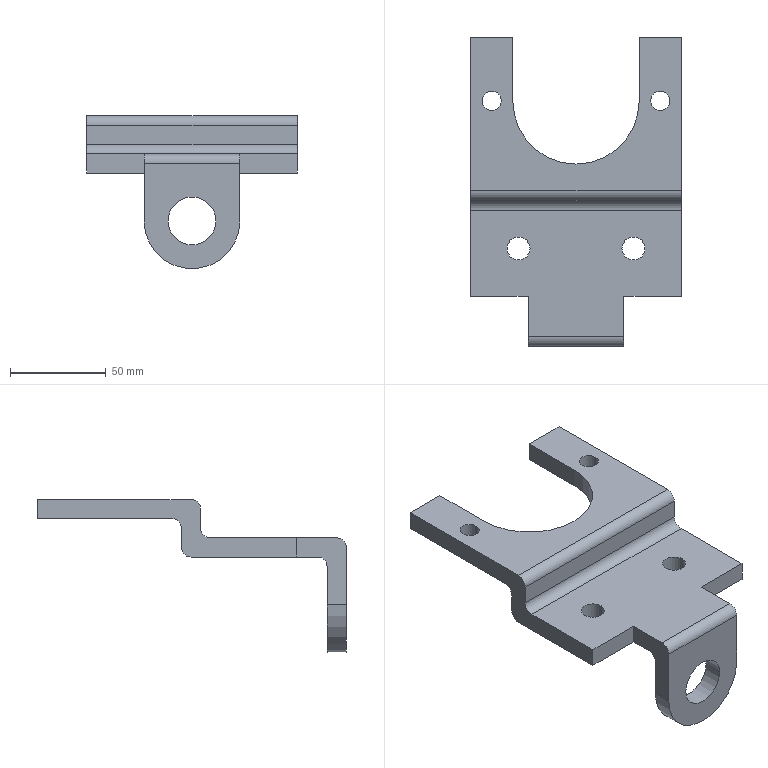Part | SolidWorks | features ICE 4, Fillet 2, Extrusion 1 | 1 solid | 36 faces | box 110 x 161 x 80 mm | volume 158190 mm3 | cylinder 18 | plane 18 | commonest cylinder face diameters 10 x10 12 x4 25 x2 50 x1 66 x1
STEP:
#1=CARTESIAN_POINT('',(-49.,102.,30.));
#2=VERTEX_POINT('',#1);
#3=CARTESIAN_POINT('',(-39.,102.,30.));
#4=VERTEX_POINT('',#3);
#5=CARTESIAN_POINT('',(-44.,102.,30.));
#6=DIRECTION('',(0.,0.,1.));
#7=DIRECTION('',(1.,0.,0.));
#8=AXIS2_PLACEMENT_3D('',#5,#6,#7);
#9=CIRCLE('',#8,5.);
#10=EDGE_CURVE('',#2,#4,#9,.T.);
#11=ORIENTED_EDGE('',*,*,#10,.T.);
#12=CARTESIAN_POINT('',(-39.,102.,20.));
#13=VERTEX_POINT('',#12);
#14=CARTESIAN_POINT('',(-39.,102.,30.));
#15=DIRECTION('',(0.,0.,-1.));
#16=VECTOR('',#15,1000.);
#17=LINE('',#14,#16);
#18=EDGE_CURVE('',#4,#13,#17,.T.);
#19=ORIENTED_EDGE('',*,*,#18,.T.);
#20=CARTESIAN_POINT('',(-49.,102.,20.));
#21=VERTEX_POINT('',#20);
#22=CARTESIAN_POINT('',(-44.,102.,20.));
#23=DIRECTION('',(0.,0.,1.));
#24=DIRECTION('',(1.,0.,0.));
#25=AXIS2_PLACEMENT_3D('',#22,#23,#24);
#26=CIRCLE('',#25,5.);
#27=EDGE_CURVE('',#21,#13,#26,.T.);
#28=ORIENTED_EDGE('',*,*,#27,.F.);
#29=CARTESIAN_POINT('',(-49.,102.,30.));
#30=DIRECTION('',(0.,0.,-1.));
#31=VECTOR('',#30,1000.);
#32=LINE('',#29,#31);
#33=EDGE_CURVE('',#2,#21,#32,.T.);
#34=ORIENTED_EDGE('',*,*,#33,.F.);
#35=EDGE_LOOP('',(#11,#19,#28,#34));
#36=FACE_OUTER_BOUND('',#35,.T.);
#37=CARTESIAN_POINT('',(-44.,102.,30.));
#38=DIRECTION('',(0.,0.,-1.));
#39=DIRECTION('',(-1.,0.,0.));
#40=AXIS2_PLACEMENT_3D('',#37,#38,#39);
#41=CYLINDRICAL_SURFACE('',#40,5.);
#42=ADVANCED_FACE('',(#36),#41,.F.);
#43=CARTESIAN_POINT('',(39.,102.,30.));
#44=VERTEX_POINT('',#43);
#45=CARTESIAN_POINT('',(49.,102.,30.));
#46=VERTEX_POINT('',#45);
#47=CARTESIAN_POINT('',(44.,102.,30.));
#48=DIRECTION('',(0.,0.,1.));
#49=DIRECTION('',(1.,0.,0.));
#50=AXIS2_PLACEMENT_3D('',#47,#48,#49);
#51=CIRCLE('',#50,5.);
#52=EDGE_CURVE('',#44,#46,#51,.T.);
#53=ORIENTED_EDGE('',*,*,#52,.T.);
#54=CARTESIAN_POINT('',(49.,102.,20.));
#55=VERTEX_POINT('',#54);
#56=CARTESIAN_POINT('',(49.,102.,30.));
#57=DIRECTION('',(0.,0.,-1.));
#58=VECTOR('',#57,1000.);
#59=LINE('',#56,#58);
#60=EDGE_CURVE('',#46,#55,#59,.T.);
#61=ORIENTED_EDGE('',*,*,#60,.T.);
#62=CARTESIAN_POINT('',(39.,102.,20.));
#63=VERTEX_POINT('',#62);
#64=CARTESIAN_POINT('',(44.,102.,20.));
#65=DIRECTION('',(0.,0.,1.));
#66=DIRECTION('',(1.,0.,0.));
#67=AXIS2_PLACEMENT_3D('',#64,#65,#66);
#68=CIRCLE('',#67,5.);
#69=EDGE_CURVE('',#63,#55,#68,.T.);
#70=ORIENTED_EDGE('',*,*,#69,.F.);
#71=CARTESIAN_POINT('',(39.,102.,30.));
#72=DIRECTION('',(0.,0.,-1.));
#73=VECTOR('',#72,1000.);
#74=LINE('',#71,#73);
#75=EDGE_CURVE('',#44,#63,#74,.T.);
#76=ORIENTED_EDGE('',*,*,#75,.F.);
#77=EDGE_LOOP('',(#53,#61,#70,#76));
#78=FACE_OUTER_BOUND('',#77,.T.);
#79=CARTESIAN_POINT('',(44.,102.,30.));
#80=DIRECTION('',(0.,0.,-1.));
#81=DIRECTION('',(-1.,0.,0.));
#82=AXIS2_PLACEMENT_3D('',#79,#80,#81);
#83=CYLINDRICAL_SURFACE('',#82,5.);
#84=ADVANCED_FACE('',(#78),#83,.F.);
#85=CARTESIAN_POINT('',(12.5,-26.,-25.));
#86=VERTEX_POINT('',#85);
#87=CARTESIAN_POINT('',(-12.5,-26.,-25.));
#88=VERTEX_POINT('',#87);
#89=CARTESIAN_POINT('',(0.,-26.,-25.));
#90=DIRECTION('',(0.,1.,0.));
#91=DIRECTION('',(-1.,0.,0.));
#92=AXIS2_PLACEMENT_3D('',#89,#90,#91);
#93=CIRCLE('',#92,12.5);
#94=EDGE_CURVE('',#86,#88,#93,.T.);
#95=ORIENTED_EDGE('',*,*,#94,.F.);
#96=CARTESIAN_POINT('',(12.5,-16.,-25.));
#97=VERTEX_POINT('',#96);
#98=CARTESIAN_POINT('',(12.5,-26.,-25.));
#99=DIRECTION('',(0.,1.,0.));
#100=VECTOR('',#99,1000.);
#101=LINE('',#98,#100);
#102=EDGE_CURVE('',#86,#97,#101,.T.);
#103=ORIENTED_EDGE('',*,*,#102,.T.);
#104=CARTESIAN_POINT('',(-12.5,-16.,-25.));
#105=VERTEX_POINT('',#104);
#106=CARTESIAN_POINT('',(0.,-16.,-25.));
#107=DIRECTION('',(0.,1.,0.));
#108=DIRECTION('',(-1.,0.,0.));
#109=AXIS2_PLACEMENT_3D('',#106,#107,#108);
#110=CIRCLE('',#109,12.5);
#111=EDGE_CURVE('',#97,#105,#110,.T.);
#112=ORIENTED_EDGE('',*,*,#111,.T.);
#113=CARTESIAN_POINT('',(-12.5,-26.,-25.));
#114=DIRECTION('',(0.,1.,0.));
#115=VECTOR('',#114,1000.);
#116=LINE('',#113,#115);
#117=EDGE_CURVE('',#88,#105,#116,.T.);
#118=ORIENTED_EDGE('',*,*,#117,.F.);
#119=EDGE_LOOP('',(#95,#103,#112,#118));
#120=FACE_OUTER_BOUND('',#119,.T.);
#121=CARTESIAN_POINT('',(0.,-26.,-25.));
#122=DIRECTION('',(0.,1.,0.));
#123=DIRECTION('',(-1.,0.,0.));
#124=AXIS2_PLACEMENT_3D('',#121,#122,#123);
#125=CYLINDRICAL_SURFACE('',#124,12.5);
#126=ADVANCED_FACE('',(#120),#125,.F.);
#127=CARTESIAN_POINT('',(24.,25.,10.));
#128=VERTEX_POINT('',#127);
#129=CARTESIAN_POINT('',(36.,25.,10.));
#130=VERTEX_POINT('',#129);
#131=CARTESIAN_POINT('',(30.,25.,10.));
#132=DIRECTION('',(0.,0.,1.));
#133=DIRECTION('',(1.,0.,0.));
#134=AXIS2_PLACEMENT_3D('',#131,#132,#133);
#135=CIRCLE('',#134,6.);
#136=EDGE_CURVE('',#128,#130,#135,.T.);
#137=ORIENTED_EDGE('',*,*,#136,.T.);
#138=CARTESIAN_POINT('',(36.,25.,0.));
#139=VERTEX_POINT('',#138);
#140=CARTESIAN_POINT('',(36.,25.,10.));
#141=DIRECTION('',(0.,0.,-1.));
#142=VECTOR('',#141,1000.);
#143=LINE('',#140,#142);
#144=EDGE_CURVE('',#130,#139,#143,.T.);
#145=ORIENTED_EDGE('',*,*,#144,.T.);
#146=CARTESIAN_POINT('',(24.,25.,0.));
#147=VERTEX_POINT('',#146);
#148=CARTESIAN_POINT('',(30.,25.,0.));
#149=DIRECTION('',(0.,0.,1.));
#150=DIRECTION('',(1.,0.,0.));
#151=AXIS2_PLACEMENT_3D('',#148,#149,#150);
#152=CIRCLE('',#151,6.);
#153=EDGE_CURVE('',#147,#139,#152,.T.);
#154=ORIENTED_EDGE('',*,*,#153,.F.);
#155=CARTESIAN_POINT('',(24.,25.,10.));
#156=DIRECTION('',(0.,0.,-1.));
#157=VECTOR('',#156,1000.);
#158=LINE('',#155,#157);
#159=EDGE_CURVE('',#128,#147,#158,.T.);
#160=ORIENTED_EDGE('',*,*,#159,.F.);
#161=EDGE_LOOP('',(#137,#145,#154,#160));
#162=FACE_OUTER_BOUND('',#161,.T.);
#163=CARTESIAN_POINT('',(30.,25.,10.));
#164=DIRECTION('',(0.,0.,-1.));
#165=DIRECTION('',(-1.,0.,0.));
#166=AXIS2_PLACEMENT_3D('',#163,#164,#165);
#167=CYLINDRICAL_SURFACE('',#166,6.);
#168=ADVANCED_FACE('',(#162),#167,.F.);
#169=CARTESIAN_POINT('',(-36.,25.,10.));
#170=VERTEX_POINT('',#169);
#171=CARTESIAN_POINT('',(-24.,25.,10.));
#172=VERTEX_POINT('',#171);
#173=CARTESIAN_POINT('',(-30.,25.,10.));
#174=DIRECTION('',(0.,0.,1.));
#175=DIRECTION('',(1.,0.,0.));
#176=AXIS2_PLACEMENT_3D('',#173,#174,#175);
#177=CIRCLE('',#176,6.);
#178=EDGE_CURVE('',#170,#172,#177,.T.);
#179=ORIENTED_EDGE('',*,*,#178,.T.);
#180=CARTESIAN_POINT('',(-24.,25.,0.));
#181=VERTEX_POINT('',#180);
#182=CARTESIAN_POINT('',(-24.,25.,10.));
#183=DIRECTION('',(0.,0.,-1.));
#184=VECTOR('',#183,1000.);
#185=LINE('',#182,#184);
#186=EDGE_CURVE('',#172,#181,#185,.T.);
#187=ORIENTED_EDGE('',*,*,#186,.T.);
#188=CARTESIAN_POINT('',(-36.,25.,0.));
#189=VERTEX_POINT('',#188);
#190=CARTESIAN_POINT('',(-30.,25.,0.));
#191=DIRECTION('',(0.,0.,1.));
#192=DIRECTION('',(1.,0.,0.));
#193=AXIS2_PLACEMENT_3D('',#190,#191,#192);
#194=CIRCLE('',#193,6.);
#195=EDGE_CURVE('',#189,#181,#194,.T.);
#196=ORIENTED_EDGE('',*,*,#195,.F.);
#197=CARTESIAN_POINT('',(-36.,25.,10.));
#198=DIRECTION('',(0.,0.,-1.));
#199=VECTOR('',#198,1000.);
#200=LINE('',#197,#199);
#201=EDGE_CURVE('',#170,#189,#200,.T.);
#202=ORIENTED_EDGE('',*,*,#201,.F.);
#203=EDGE_LOOP('',(#179,#187,#196,#202));
#204=FACE_OUTER_BOUND('',#203,.T.);
#205=CARTESIAN_POINT('',(-30.,25.,10.));
#206=DIRECTION('',(0.,0.,-1.));
#207=DIRECTION('',(-1.,0.,0.));
#208=AXIS2_PLACEMENT_3D('',#205,#206,#207);
#209=CYLINDRICAL_SURFACE('',#208,6.);
#210=ADVANCED_FACE('',(#204),#209,.F.);
#211=CARTESIAN_POINT('',(25.,-21.,10.));
#212=VERTEX_POINT('',#211);
#213=CARTESIAN_POINT('',(25.,0.,10.));
#214=VERTEX_POINT('',#213);
#215=CARTESIAN_POINT('',(25.,-16.,10.));
#216=DIRECTION('',(0.,1.,0.));
#217=VECTOR('',#216,1000.);
#218=LINE('',#215,#217);
#219=EDGE_CURVE('',#212,#214,#218,.T.);
#220=ORIENTED_EDGE('',*,*,#219,.F.);
#221=CARTESIAN_POINT('',(25.,-26.,5.));
#222=VERTEX_POINT('',#221);
#223=CARTESIAN_POINT('',(25.,-21.,5.));
#224=DIRECTION('',(1.,0.,0.));
#225=DIRECTION('',(0.,0.,1.));
#226=AXIS2_PLACEMENT_3D('',#223,#224,#225);
#227=CIRCLE('',#226,5.);
#228=EDGE_CURVE('',#212,#222,#227,.T.);
#229=ORIENTED_EDGE('',*,*,#228,.T.);
#230=CARTESIAN_POINT('',(25.,-26.,-25.));
#231=VERTEX_POINT('',#230);
#232=CARTESIAN_POINT('',(25.,-26.,-50.));
#233=DIRECTION('',(0.,0.,1.));
#234=VECTOR('',#233,1000.);
#235=LINE('',#232,#234);
#236=EDGE_CURVE('',#231,#222,#235,.T.);
#237=ORIENTED_EDGE('',*,*,#236,.F.);
#238=CARTESIAN_POINT('',(25.,-16.,-25.));
#239=VERTEX_POINT('',#238);
#240=CARTESIAN_POINT('',(25.,-26.,-25.));
#241=DIRECTION('',(0.,1.,0.));
#242=VECTOR('',#241,1000.);
#243=LINE('',#240,#242);
#244=EDGE_CURVE('',#231,#239,#243,.T.);
#245=ORIENTED_EDGE('',*,*,#244,.T.);
#246=CARTESIAN_POINT('',(25.,-16.,-5.));
#247=VERTEX_POINT('',#246);
#248=CARTESIAN_POINT('',(25.,-16.,-50.));
#249=DIRECTION('',(0.,0.,1.));
#250=VECTOR('',#249,1000.);
#251=LINE('',#248,#250);
#252=EDGE_CURVE('',#239,#247,#251,.T.);
#253=ORIENTED_EDGE('',*,*,#252,.T.);
#254=CARTESIAN_POINT('',(25.,-11.,0.));
#255=VERTEX_POINT('',#254);
#256=CARTESIAN_POINT('',(25.,-11.,-5.));
#257=DIRECTION('',(-1.,0.,0.));
#258=DIRECTION('',(0.,0.,1.));
#259=AXIS2_PLACEMENT_3D('',#256,#257,#258);
#260=CIRCLE('',#259,5.);
#261=EDGE_CURVE('',#247,#255,#260,.T.);
#262=ORIENTED_EDGE('',*,*,#261,.T.);
#263=CARTESIAN_POINT('',(25.,0.,0.));
#264=VERTEX_POINT('',#263);
#265=CARTESIAN_POINT('',(25.,-16.,0.));
#266=DIRECTION('',(0.,1.,0.));
#267=VECTOR('',#266,1000.);
#268=LINE('',#265,#267);
#269=EDGE_CURVE('',#255,#264,#268,.T.);
#270=ORIENTED_EDGE('',*,*,#269,.T.);
#271=CARTESIAN_POINT('',(25.,0.,10.));
#272=DIRECTION('',(0.,0.,-1.));
#273=VECTOR('',#272,1000.);
#274=LINE('',#271,#273);
#275=EDGE_CURVE('',#214,#264,#274,.T.);
#276=ORIENTED_EDGE('',*,*,#275,.F.);
#277=EDGE_LOOP('',(#220,#229,#237,#245,#253,#262,#270,#276));
#278=FACE_OUTER_BOUND('',#277,.T.);
#279=CARTESIAN_POINT('',(25.,-16.,10.));
#280=DIRECTION('',(-1.,0.,0.));
#281=DIRECTION('',(0.,0.,1.));
#282=AXIS2_PLACEMENT_3D('',#279,#280,#281);
#283=PLANE('',#282);
#284=ADVANCED_FACE('',(#278),#283,.F.);
#285=ORIENTED_EDGE('',*,*,#178,.F.);
#286=CARTESIAN_POINT('',(-30.,25.,10.));
#287=DIRECTION('',(0.,0.,1.));
#288=DIRECTION('',(1.,0.,0.));
#289=AXIS2_PLACEMENT_3D('',#286,#287,#288);
#290=CIRCLE('',#289,6.);
#291=EDGE_CURVE('',#172,#170,#290,.T.);
#292=ORIENTED_EDGE('',*,*,#291,.F.);
#293=EDGE_LOOP('',(#285,#292));
#294=FACE_BOUND('',#293,.T.);
#295=CARTESIAN_POINT('',(55.,0.,10.));
#296=VERTEX_POINT('',#295);
#297=CARTESIAN_POINT('',(55.,45.,10.));
#298=VERTEX_POINT('',#297);
#299=CARTESIAN_POINT('',(55.,50.,10.));
#300=DIRECTION('',(0.,1.,0.));
#301=VECTOR('',#300,1000.);
#302=LINE('',#299,#301);
#303=EDGE_CURVE('',#296,#298,#302,.T.);
#304=ORIENTED_EDGE('',*,*,#303,.T.);
#305=CARTESIAN_POINT('',(-55.,45.,10.));
#306=VERTEX_POINT('',#305);
#307=CARTESIAN_POINT('',(0.,45.,10.));
#308=DIRECTION('',(-1.,0.,0.));
#309=VECTOR('',#308,1000.);
#310=LINE('',#307,#309);
#311=EDGE_CURVE('',#298,#306,#310,.T.);
#312=ORIENTED_EDGE('',*,*,#311,.T.);
#313=CARTESIAN_POINT('',(-55.,0.,10.));
#314=VERTEX_POINT('',#313);
#315=CARTESIAN_POINT('',(-55.,50.,10.));
#316=DIRECTION('',(0.,-1.,0.));
#317=VECTOR('',#316,1000.);
#318=LINE('',#315,#317);
#319=EDGE_CURVE('',#306,#314,#318,.T.);
#320=ORIENTED_EDGE('',*,*,#319,.T.);
#321=CARTESIAN_POINT('',(-25.,0.,10.));
#322=VERTEX_POINT('',#321);
#323=CARTESIAN_POINT('',(-55.,0.,10.));
#324=DIRECTION('',(1.,0.,0.));
#325=VECTOR('',#324,1000.);
#326=LINE('',#323,#325);
#327=EDGE_CURVE('',#314,#322,#326,.T.);
#328=ORIENTED_EDGE('',*,*,#327,.T.);
#329=CARTESIAN_POINT('',(-25.,-21.,10.));
#330=VERTEX_POINT('',#329);
#331=CARTESIAN_POINT('',(-25.,0.,10.));
#332=DIRECTION('',(0.,-1.,0.));
#333=VECTOR('',#332,1000.);
#334=LINE('',#331,#333);
#335=EDGE_CURVE('',#322,#330,#334,.T.);
#336=ORIENTED_EDGE('',*,*,#335,.T.);
#337=CARTESIAN_POINT('',(25.,-21.,10.));
#338=DIRECTION('',(1.,0.,0.));
#339=VECTOR('',#338,1000.);
#340=LINE('',#337,#339);
#341=EDGE_CURVE('',#330,#212,#340,.T.);
#342=ORIENTED_EDGE('',*,*,#341,.T.);
#343=ORIENTED_EDGE('',*,*,#219,.T.);
#344=CARTESIAN_POINT('',(55.,0.,10.));
#345=DIRECTION('',(1.,0.,0.));
#346=VECTOR('',#345,1000.);
#347=LINE('',#344,#346);
#348=EDGE_CURVE('',#214,#296,#347,.T.);
#349=ORIENTED_EDGE('',*,*,#348,.T.);
#350=EDGE_LOOP('',(#304,#312,#320,#328,#336,#342,#343,#349));
#351=FACE_OUTER_BOUND('',#350,.T.);
#352=ORIENTED_EDGE('',*,*,#136,.F.);
#353=CARTESIAN_POINT('',(30.,25.,10.));
#354=DIRECTION('',(0.,0.,1.));
#355=DIRECTION('',(1.,0.,0.));
#356=AXIS2_PLACEMENT_3D('',#353,#354,#355);
#357=CIRCLE('',#356,6.);
#358=EDGE_CURVE('',#130,#128,#357,.T.);
#359=ORIENTED_EDGE('',*,*,#358,.F.);
#360=EDGE_LOOP('',(#352,#359));
#361=FACE_BOUND('',#360,.T.);
#362=CARTESIAN_POINT('',(0.,0.,10.));
#363=DIRECTION('',(0.,0.,-1.));
#364=DIRECTION('',(-1.,0.,0.));
#365=AXIS2_PLACEMENT_3D('',#362,#363,#364);
#366=PLANE('',#365);
#367=ADVANCED_FACE('',(#294,#351,#361),#366,.F.);
#368=ORIENTED_EDGE('',*,*,#195,.T.);
#369=CARTESIAN_POINT('',(-30.,25.,0.));
#370=DIRECTION('',(0.,0.,1.));
#371=DIRECTION('',(1.,0.,0.));
#372=AXIS2_PLACEMENT_3D('',#369,#370,#371);
#373=CIRCLE('',#372,6.);
#374=EDGE_CURVE('',#181,#189,#373,.T.);
#375=ORIENTED_EDGE('',*,*,#374,.T.);
#376=EDGE_LOOP('',(#368,#375));
#377=FACE_BOUND('',#376,.T.);
#378=CARTESIAN_POINT('',(-55.,55.,0.));
#379=VERTEX_POINT('',#378);
#380=CARTESIAN_POINT('',(-55.,0.,0.));
#381=VERTEX_POINT('',#380);
#382=CARTESIAN_POINT('',(-55.,50.,0.));
#383=DIRECTION('',(0.,-1.,0.));
#384=VECTOR('',#383,1000.);
#385=LINE('',#382,#384);
#386=EDGE_CURVE('',#379,#381,#385,.T.);
#387=ORIENTED_EDGE('',*,*,#386,.F.);
#388=CARTESIAN_POINT('',(55.,55.,0.));
#389=VERTEX_POINT('',#388);
#390=CARTESIAN_POINT('',(0.,55.,0.));
#391=DIRECTION('',(1.,0.,0.));
#392=VECTOR('',#391,1000.);
#393=LINE('',#390,#392);
#394=EDGE_CURVE('',#379,#389,#393,.T.);
#395=ORIENTED_EDGE('',*,*,#394,.T.);
#396=CARTESIAN_POINT('',(55.,0.,0.));
#397=VERTEX_POINT('',#396);
#398=CARTESIAN_POINT('',(55.,50.,0.));
#399=DIRECTION('',(0.,1.,0.));
#400=VECTOR('',#399,1000.);
#401=LINE('',#398,#400);
#402=EDGE_CURVE('',#397,#389,#401,.T.);
#403=ORIENTED_EDGE('',*,*,#402,.F.);
#404=CARTESIAN_POINT('',(25.,0.,0.));
#405=DIRECTION('',(1.,0.,0.));
#406=VECTOR('',#405,1000.);
#407=LINE('',#404,#406);
#408=EDGE_CURVE('',#264,#397,#407,.T.);
#409=ORIENTED_EDGE('',*,*,#408,.F.);
#410=ORIENTED_EDGE('',*,*,#269,.F.);
#411=CARTESIAN_POINT('',(-25.,-11.,0.));
#412=VERTEX_POINT('',#411);
#413=CARTESIAN_POINT('',(-25.,-11.,0.));
#414=DIRECTION('',(-1.,0.,0.));
#415=VECTOR('',#414,1000.);
#416=LINE('',#413,#415);
#417=EDGE_CURVE('',#255,#412,#416,.T.);
#418=ORIENTED_EDGE('',*,*,#417,.T.);
#419=CARTESIAN_POINT('',(-25.,0.,0.));
#420=VERTEX_POINT('',#419);
#421=CARTESIAN_POINT('',(-25.,0.,0.));
#422=DIRECTION('',(0.,-1.,0.));
#423=VECTOR('',#422,1000.);
#424=LINE('',#421,#423);
#425=EDGE_CURVE('',#420,#412,#424,.T.);
#426=ORIENTED_EDGE('',*,*,#425,.F.);
#427=CARTESIAN_POINT('',(-55.,0.,0.));
#428=DIRECTION('',(1.,0.,0.));
#429=VECTOR('',#428,1000.);
#430=LINE('',#427,#429);
#431=EDGE_CURVE('',#381,#420,#430,.T.);
#432=ORIENTED_EDGE('',*,*,#431,.F.);
#433=EDGE_LOOP('',(#387,#395,#403,#409,#410,#418,#426,#432));
#434=FACE_OUTER_BOUND('',#433,.T.);
#435=ORIENTED_EDGE('',*,*,#153,.T.);
#436=CARTESIAN_POINT('',(30.,25.,0.));
#437=DIRECTION('',(0.,0.,1.));
#438=DIRECTION('',(1.,0.,0.));
#439=AXIS2_PLACEMENT_3D('',#436,#437,#438);
#440=CIRCLE('',#439,6.);
#441=EDGE_CURVE('',#139,#147,#440,.T.);
#442=ORIENTED_EDGE('',*,*,#441,.T.);
#443=EDGE_LOOP('',(#435,#442));
#444=FACE_BOUND('',#443,.T.);
#445=CARTESIAN_POINT('',(0.,0.,0.));
#446=DIRECTION('',(0.,0.,-1.));
#447=DIRECTION('',(-1.,0.,0.));
#448=AXIS2_PLACEMENT_3D('',#445,#446,#447);
#449=PLANE('',#448);
#450=ADVANCED_FACE('',(#377,#434,#444),#449,.T.);
#451=CARTESIAN_POINT('',(55.,55.,30.));
#452=VERTEX_POINT('',#451);
#453=CARTESIAN_POINT('',(55.,135.,30.));
#454=VERTEX_POINT('',#453);
#455=CARTESIAN_POINT('',(55.,50.,30.));
#456=DIRECTION('',(0.,1.,0.));
#457=VECTOR('',#456,1000.);
#458=LINE('',#455,#457);
#459=EDGE_CURVE('',#452,#454,#458,.T.);
#460=ORIENTED_EDGE('',*,*,#459,.F.);
#461=CARTESIAN_POINT('',(55.,50.,25.));
#462=VERTEX_POINT('',#461);
#463=CARTESIAN_POINT('',(55.,55.,25.));
#464=DIRECTION('',(1.,0.,0.));
#465=DIRECTION('',(0.,-1.,0.));
#466=AXIS2_PLACEMENT_3D('',#463,#464,#465);
#467=CIRCLE('',#466,5.);
#468=EDGE_CURVE('',#452,#462,#467,.T.);
#469=ORIENTED_EDGE('',*,*,#468,.T.);
#470=CARTESIAN_POINT('',(55.,50.,15.));
#471=VERTEX_POINT('',#470);
#472=CARTESIAN_POINT('',(55.,50.,0.));
#473=DIRECTION('',(0.,0.,1.));
#474=VECTOR('',#473,1000.);
#475=LINE('',#472,#474);
#476=EDGE_CURVE('',#471,#462,#475,.T.);
#477=ORIENTED_EDGE('',*,*,#476,.F.);
#478=CARTESIAN_POINT('',(55.,45.,15.));
#479=DIRECTION('',(-1.,0.,0.));
#480=DIRECTION('',(0.,-1.,0.));
#481=AXIS2_PLACEMENT_3D('',#478,#479,#480);
#482=CIRCLE('',#481,5.);
#483=EDGE_CURVE('',#471,#298,#482,.T.);
#484=ORIENTED_EDGE('',*,*,#483,.T.);
#485=ORIENTED_EDGE('',*,*,#303,.F.);
#486=CARTESIAN_POINT('',(55.,0.,10.));
#487=DIRECTION('',(0.,0.,-1.));
#488=VECTOR('',#487,1000.);
#489=LINE('',#486,#488);
#490=EDGE_CURVE('',#296,#397,#489,.T.);
#491=ORIENTED_EDGE('',*,*,#490,.T.);
#492=ORIENTED_EDGE('',*,*,#402,.T.);
#493=CARTESIAN_POINT('',(55.,60.,5.));
#494=VERTEX_POINT('',#493);
#495=CARTESIAN_POINT('',(55.,55.,5.));
#496=DIRECTION('',(1.,0.,0.));
#497=DIRECTION('',(0.,-1.,0.));
#498=AXIS2_PLACEMENT_3D('',#495,#496,#497);
#499=CIRCLE('',#498,5.);
#500=EDGE_CURVE('',#389,#494,#499,.T.);
#501=ORIENTED_EDGE('',*,*,#500,.T.);
#502=CARTESIAN_POINT('',(55.,60.,15.));
#503=VERTEX_POINT('',#502);
#504=CARTESIAN_POINT('',(55.,60.,0.));
#505=DIRECTION('',(0.,0.,1.));
#506=VECTOR('',#505,1000.);
#507=LINE('',#504,#506);
#508=EDGE_CURVE('',#494,#503,#507,.T.);
#509=ORIENTED_EDGE('',*,*,#508,.T.);
#510=CARTESIAN_POINT('',(55.,65.,20.));
#511=VERTEX_POINT('',#510);
#512=CARTESIAN_POINT('',(55.,65.,15.));
#513=DIRECTION('',(-1.,0.,0.));
#514=DIRECTION('',(0.,-1.,0.));
#515=AXIS2_PLACEMENT_3D('',#512,#513,#514);
#516=CIRCLE('',#515,5.);
#517=EDGE_CURVE('',#503,#511,#516,.T.);
#518=ORIENTED_EDGE('',*,*,#517,.T.);
#519=CARTESIAN_POINT('',(55.,135.,20.));
#520=VERTEX_POINT('',#519);
#521=CARTESIAN_POINT('',(55.,60.,20.));
#522=DIRECTION('',(0.,1.,0.));
#523=VECTOR('',#522,1000.);
#524=LINE('',#521,#523);
#525=EDGE_CURVE('',#511,#520,#524,.T.);
#526=ORIENTED_EDGE('',*,*,#525,.T.);
#527=CARTESIAN_POINT('',(55.,135.,30.));
#528=DIRECTION('',(0.,0.,-1.));
#529=VECTOR('',#528,1000.);
#530=LINE('',#527,#529);
#531=EDGE_CURVE('',#454,#520,#530,.T.);
#532=ORIENTED_EDGE('',*,*,#531,.F.);
#533=EDGE_LOOP('',(#460,#469,#477,#484,#485,#491,#492,#501,#509,#518,#526,#532));
#534=FACE_OUTER_BOUND('',#533,.T.);
#535=CARTESIAN_POINT('',(55.,50.,10.));
#536=DIRECTION('',(-1.,0.,0.));
#537=DIRECTION('',(0.,-1.,0.));
#538=AXIS2_PLACEMENT_3D('',#535,#536,#537);
#539=PLANE('',#538);
#540=ADVANCED_FACE('',(#534),#539,.F.);
#541=CARTESIAN_POINT('',(-55.,50.,15.));
#542=VERTEX_POINT('',#541);
#543=CARTESIAN_POINT('',(-55.,50.,25.));
#544=VERTEX_POINT('',#543);
#545=CARTESIAN_POINT('',(-55.,50.,0.));
#546=DIRECTION('',(0.,0.,1.));
#547=VECTOR('',#546,1000.);
#548=LINE('',#545,#547);
#549=EDGE_CURVE('',#542,#544,#548,.T.);
#550=ORIENTED_EDGE('',*,*,#549,.T.);
#551=CARTESIAN_POINT('',(-55.,55.,30.));
#552=VERTEX_POINT('',#551);
#553=CARTESIAN_POINT('',(-55.,55.,25.));
#554=DIRECTION('',(-1.,0.,0.));
#555=DIRECTION('',(0.,1.,0.));
#556=AXIS2_PLACEMENT_3D('',#553,#554,#555);
#557=CIRCLE('',#556,5.);
#558=EDGE_CURVE('',#544,#552,#557,.T.);
#559=ORIENTED_EDGE('',*,*,#558,.T.);
#560=CARTESIAN_POINT('',(-55.,135.,30.));
#561=VERTEX_POINT('',#560);
#562=CARTESIAN_POINT('',(-55.,60.,30.));
#563=DIRECTION('',(0.,-1.,0.));
#564=VECTOR('',#563,1000.);
#565=LINE('',#562,#564);
#566=EDGE_CURVE('',#561,#552,#565,.T.);
#567=ORIENTED_EDGE('',*,*,#566,.F.);
#568=CARTESIAN_POINT('',(-55.,135.,20.));
#569=VERTEX_POINT('',#568);
#570=CARTESIAN_POINT('',(-55.,135.,30.));
#571=DIRECTION('',(0.,0.,-1.));
#572=VECTOR('',#571,1000.);
#573=LINE('',#570,#572);
#574=EDGE_CURVE('',#561,#569,#573,.T.);
#575=ORIENTED_EDGE('',*,*,#574,.T.);
#576=CARTESIAN_POINT('',(-55.,65.,20.));
#577=VERTEX_POINT('',#576);
#578=CARTESIAN_POINT('',(-55.,60.,20.));
#579=DIRECTION('',(0.,-1.,0.));
#580=VECTOR('',#579,1000.);
#581=LINE('',#578,#580);
#582=EDGE_CURVE('',#569,#577,#581,.T.);
#583=ORIENTED_EDGE('',*,*,#582,.T.);
#584=CARTESIAN_POINT('',(-55.,60.,15.));
#585=VERTEX_POINT('',#584);
#586=CARTESIAN_POINT('',(-55.,65.,15.));
#587=DIRECTION('',(1.,0.,0.));
#588=DIRECTION('',(0.,1.,0.));
#589=AXIS2_PLACEMENT_3D('',#586,#587,#588);
#590=CIRCLE('',#589,5.);
#591=EDGE_CURVE('',#577,#585,#590,.T.);
#592=ORIENTED_EDGE('',*,*,#591,.T.);
#593=CARTESIAN_POINT('',(-55.,60.,5.));
#594=VERTEX_POINT('',#593);
#595=CARTESIAN_POINT('',(-55.,60.,0.));
#596=DIRECTION('',(0.,0.,1.));
#597=VECTOR('',#596,1000.);
#598=LINE('',#595,#597);
#599=EDGE_CURVE('',#594,#585,#598,.T.);
#600=ORIENTED_EDGE('',*,*,#599,.F.);
#601=CARTESIAN_POINT('',(-55.,55.,5.));
#602=DIRECTION('',(-1.,0.,0.));
#603=DIRECTION('',(0.,1.,0.));
#604=AXIS2_PLACEMENT_3D('',#601,#602,#603);
#605=CIRCLE('',#604,5.);
#606=EDGE_CURVE('',#594,#379,#605,.T.);
#607=ORIENTED_EDGE('',*,*,#606,.T.);
#608=ORIENTED_EDGE('',*,*,#386,.T.);
#609=CARTESIAN_POINT('',(-55.,0.,10.));
#610=DIRECTION('',(0.,0.,-1.));
#611=VECTOR('',#610,1000.);
#612=LINE('',#609,#611);
#613=EDGE_CURVE('',#314,#381,#612,.T.);
#614=ORIENTED_EDGE('',*,*,#613,.F.);
#615=ORIENTED_EDGE('',*,*,#319,.F.);
#616=CARTESIAN_POINT('',(-55.,45.,15.));
#617=DIRECTION('',(1.,0.,0.));
#618=DIRECTION('',(0.,1.,0.));
#619=AXIS2_PLACEMENT_3D('',#616,#617,#618);
#620=CIRCLE('',#619,5.);
#621=EDGE_CURVE('',#306,#542,#620,.T.);
#622=ORIENTED_EDGE('',*,*,#621,.T.);
#623=EDGE_LOOP('',(#550,#559,#567,#575,#583,#592,#600,#607,#608,#614,#615,#622));
#624=FACE_OUTER_BOUND('',#623,.T.);
#625=CARTESIAN_POINT('',(-55.,50.,10.));
#626=DIRECTION('',(1.,0.,0.));
#627=DIRECTION('',(0.,1.,0.));
#628=AXIS2_PLACEMENT_3D('',#625,#626,#627);
#629=PLANE('',#628);
#630=ADVANCED_FACE('',(#624),#629,.F.);
#631=ORIENTED_EDGE('',*,*,#431,.T.);
#632=CARTESIAN_POINT('',(-25.,0.,10.));
#633=DIRECTION('',(0.,0.,-1.));
#634=VECTOR('',#633,1000.);
#635=LINE('',#632,#634);
#636=EDGE_CURVE('',#322,#420,#635,.T.);
#637=ORIENTED_EDGE('',*,*,#636,.F.);
#638=ORIENTED_EDGE('',*,*,#327,.F.);
#639=ORIENTED_EDGE('',*,*,#613,.T.);
#640=EDGE_LOOP('',(#631,#637,#638,#639));
#641=FACE_OUTER_BOUND('',#640,.T.);
#642=CARTESIAN_POINT('',(-55.,0.,10.));
#643=DIRECTION('',(0.,1.,0.));
#644=DIRECTION('',(-1.,0.,0.));
#645=AXIS2_PLACEMENT_3D('',#642,#643,#644);
#646=PLANE('',#645);
#647=ADVANCED_FACE('',(#641),#646,.F.);
#648=CARTESIAN_POINT('',(-25.,-26.,-25.));
#649=VERTEX_POINT('',#648);
#650=CARTESIAN_POINT('',(-25.,-26.,5.));
#651=VERTEX_POINT('',#650);
#652=CARTESIAN_POINT('',(-25.,-26.,-50.));
#653=DIRECTION('',(0.,0.,1.));
#654=VECTOR('',#653,1000.);
#655=LINE('',#652,#654);
#656=EDGE_CURVE('',#649,#651,#655,.T.);
#657=ORIENTED_EDGE('',*,*,#656,.T.);
#658=CARTESIAN_POINT('',(-25.,-21.,5.));
#659=DIRECTION('',(-1.,0.,0.));
#660=DIRECTION('',(0.,1.,0.));
#661=AXIS2_PLACEMENT_3D('',#658,#659,#660);
#662=CIRCLE('',#661,5.);
#663=EDGE_CURVE('',#651,#330,#662,.T.);
#664=ORIENTED_EDGE('',*,*,#663,.T.);
#665=ORIENTED_EDGE('',*,*,#335,.F.);
#666=ORIENTED_EDGE('',*,*,#636,.T.);
#667=ORIENTED_EDGE('',*,*,#425,.T.);
#668=CARTESIAN_POINT('',(-25.,-16.,-5.));
#669=VERTEX_POINT('',#668);
#670=CARTESIAN_POINT('',(-25.,-11.,-5.));
#671=DIRECTION('',(1.,0.,0.));
#672=DIRECTION('',(0.,1.,0.));
#673=AXIS2_PLACEMENT_3D('',#670,#671,#672);
#674=CIRCLE('',#673,5.);
#675=EDGE_CURVE('',#412,#669,#674,.T.);
#676=ORIENTED_EDGE('',*,*,#675,.T.);
#677=CARTESIAN_POINT('',(-25.,-16.,-25.));
#678=VERTEX_POINT('',#677);
#679=CARTESIAN_POINT('',(-25.,-16.,-50.));
#680=DIRECTION('',(0.,0.,1.));
#681=VECTOR('',#680,1000.);
#682=LINE('',#679,#681);
#683=EDGE_CURVE('',#678,#669,#682,.T.);
#684=ORIENTED_EDGE('',*,*,#683,.F.);
#685=CARTESIAN_POINT('',(-25.,-26.,-25.));
#686=DIRECTION('',(0.,1.,0.));
#687=VECTOR('',#686,1000.);
#688=LINE('',#685,#687);
#689=EDGE_CURVE('',#649,#678,#688,.T.);
#690=ORIENTED_EDGE('',*,*,#689,.F.);
#691=EDGE_LOOP('',(#657,#664,#665,#666,#667,#676,#684,#690));
#692=FACE_OUTER_BOUND('',#691,.T.);
#693=CARTESIAN_POINT('',(-25.,0.,10.));
#694=DIRECTION('',(1.,0.,0.));
#695=DIRECTION('',(0.,1.,0.));
#696=AXIS2_PLACEMENT_3D('',#693,#694,#695);
#697=PLANE('',#696);
#698=ADVANCED_FACE('',(#692),#697,.F.);
#699=ORIENTED_EDGE('',*,*,#408,.T.);
#700=ORIENTED_EDGE('',*,*,#490,.F.);
#701=ORIENTED_EDGE('',*,*,#348,.F.);
#702=ORIENTED_EDGE('',*,*,#275,.T.);
#703=EDGE_LOOP('',(#699,#700,#701,#702));
#704=FACE_OUTER_BOUND('',#703,.T.);
#705=CARTESIAN_POINT('',(25.,0.,10.));
#706=DIRECTION('',(0.,1.,0.));
#707=DIRECTION('',(0.,0.,1.));
#708=AXIS2_PLACEMENT_3D('',#705,#706,#707);
#709=PLANE('',#708);
#710=ADVANCED_FACE('',(#704),#709,.F.);
#711=ORIENTED_EDGE('',*,*,#186,.F.);
#712=ORIENTED_EDGE('',*,*,#291,.T.);
#713=ORIENTED_EDGE('',*,*,#201,.T.);
#714=ORIENTED_EDGE('',*,*,#374,.F.);
#715=EDGE_LOOP('',(#711,#712,#713,#714));
#716=FACE_OUTER_BOUND('',#715,.T.);
#717=CARTESIAN_POINT('',(-30.,25.,10.));
#718=DIRECTION('',(0.,0.,-1.));
#719=DIRECTION('',(-1.,0.,0.));
#720=AXIS2_PLACEMENT_3D('',#717,#718,#719);
#721=CYLINDRICAL_SURFACE('',#720,6.);
#722=ADVANCED_FACE('',(#716),#721,.F.);
#723=ORIENTED_EDGE('',*,*,#144,.F.);
#724=ORIENTED_EDGE('',*,*,#358,.T.);
#725=ORIENTED_EDGE('',*,*,#159,.T.);
#726=ORIENTED_EDGE('',*,*,#441,.F.);
#727=EDGE_LOOP('',(#723,#724,#725,#726));
#728=FACE_OUTER_BOUND('',#727,.T.);
#729=CARTESIAN_POINT('',(30.,25.,10.));
#730=DIRECTION('',(0.,0.,-1.));
#731=DIRECTION('',(-1.,0.,0.));
#732=AXIS2_PLACEMENT_3D('',#729,#730,#731);
#733=CYLINDRICAL_SURFACE('',#732,6.);
#734=ADVANCED_FACE('',(#728),#733,.F.);
#735=ORIENTED_EDGE('',*,*,#236,.T.);
#736=CARTESIAN_POINT('',(-25.,-26.,5.));
#737=DIRECTION('',(-1.,0.,0.));
#738=VECTOR('',#737,1000.);
#739=LINE('',#736,#738);
#740=EDGE_CURVE('',#222,#651,#739,.T.);
#741=ORIENTED_EDGE('',*,*,#740,.T.);
#742=ORIENTED_EDGE('',*,*,#656,.F.);
#743=CARTESIAN_POINT('',(0.,-26.,-25.));
#744=DIRECTION('',(0.,-1.,0.));
#745=DIRECTION('',(-1.,0.,0.));
#746=AXIS2_PLACEMENT_3D('',#743,#744,#745);
#747=CIRCLE('',#746,25.);
#748=EDGE_CURVE('',#649,#231,#747,.T.);
#749=ORIENTED_EDGE('',*,*,#748,.T.);
#750=EDGE_LOOP('',(#735,#741,#742,#749));
#751=FACE_OUTER_BOUND('',#750,.T.);
#752=CARTESIAN_POINT('',(0.,-26.,-25.));
#753=DIRECTION('',(0.,1.,0.));
#754=DIRECTION('',(-1.,0.,0.));
#755=AXIS2_PLACEMENT_3D('',#752,#753,#754);
#756=CIRCLE('',#755,12.5);
#757=EDGE_CURVE('',#88,#86,#756,.T.);
#758=ORIENTED_EDGE('',*,*,#757,.T.);
#759=ORIENTED_EDGE('',*,*,#94,.T.);
#760=EDGE_LOOP('',(#758,#759));
#761=FACE_BOUND('',#760,.T.);
#762=CARTESIAN_POINT('',(-25.,-26.,-50.));
#763=DIRECTION('',(0.,-1.,0.));
#764=DIRECTION('',(0.,0.,-1.));
#765=AXIS2_PLACEMENT_3D('',#762,#763,#764);
#766=PLANE('',#765);
#767=ADVANCED_FACE('',(#751,#761),#766,.T.);
#768=ORIENTED_EDGE('',*,*,#683,.T.);
#769=CARTESIAN_POINT('',(25.,-16.,-5.));
#770=DIRECTION('',(1.,0.,0.));
#771=VECTOR('',#770,1000.);
#772=LINE('',#769,#771);
#773=EDGE_CURVE('',#669,#247,#772,.T.);
#774=ORIENTED_EDGE('',*,*,#773,.T.);
#775=ORIENTED_EDGE('',*,*,#252,.F.);
#776=CARTESIAN_POINT('',(0.,-16.,-25.));
#777=DIRECTION('',(0.,-1.,0.));
#778=DIRECTION('',(-1.,0.,0.));
#779=AXIS2_PLACEMENT_3D('',#776,#777,#778);
#780=CIRCLE('',#779,25.);
#781=EDGE_CURVE('',#678,#239,#780,.T.);
#782=ORIENTED_EDGE('',*,*,#781,.F.);
#783=EDGE_LOOP('',(#768,#774,#775,#782));
#784=FACE_OUTER_BOUND('',#783,.T.);
#785=CARTESIAN_POINT('',(0.,-16.,-25.));
#786=DIRECTION('',(0.,1.,0.));
#787=DIRECTION('',(-1.,0.,0.));
#788=AXIS2_PLACEMENT_3D('',#785,#786,#787);
#789=CIRCLE('',#788,12.5);
#790=EDGE_CURVE('',#105,#97,#789,.T.);
#791=ORIENTED_EDGE('',*,*,#790,.F.);
#792=ORIENTED_EDGE('',*,*,#111,.F.);
#793=EDGE_LOOP('',(#791,#792));
#794=FACE_BOUND('',#793,.T.);
#795=CARTESIAN_POINT('',(25.,-16.,-50.));
#796=DIRECTION('',(0.,1.,0.));
#797=DIRECTION('',(0.,0.,1.));
#798=AXIS2_PLACEMENT_3D('',#795,#796,#797);
#799=PLANE('',#798);
#800=ADVANCED_FACE('',(#784,#794),#799,.T.);
#801=ORIENTED_EDGE('',*,*,#102,.F.);
#802=ORIENTED_EDGE('',*,*,#757,.F.);
#803=ORIENTED_EDGE('',*,*,#117,.T.);
#804=ORIENTED_EDGE('',*,*,#790,.T.);
#805=EDGE_LOOP('',(#801,#802,#803,#804));
#806=FACE_OUTER_BOUND('',#805,.T.);
#807=CARTESIAN_POINT('',(0.,-26.,-25.));
#808=DIRECTION('',(0.,1.,0.));
#809=DIRECTION('',(-1.,0.,0.));
#810=AXIS2_PLACEMENT_3D('',#807,#808,#809);
#811=CYLINDRICAL_SURFACE('',#810,12.5);
#812=ADVANCED_FACE('',(#806),#811,.F.);
#813=ORIENTED_EDGE('',*,*,#781,.T.);
#814=ORIENTED_EDGE('',*,*,#244,.F.);
#815=ORIENTED_EDGE('',*,*,#748,.F.);
#816=ORIENTED_EDGE('',*,*,#689,.T.);
#817=EDGE_LOOP('',(#813,#814,#815,#816));
#818=FACE_OUTER_BOUND('',#817,.T.);
#819=CARTESIAN_POINT('',(0.,-26.,-25.));
#820=DIRECTION('',(0.,1.,0.));
#821=DIRECTION('',(-1.,0.,0.));
#822=AXIS2_PLACEMENT_3D('',#819,#820,#821);
#823=CYLINDRICAL_SURFACE('',#822,25.);
#824=ADVANCED_FACE('',(#818),#823,.T.);
#825=ORIENTED_EDGE('',*,*,#675,.F.);
#826=ORIENTED_EDGE('',*,*,#417,.F.);
#827=ORIENTED_EDGE('',*,*,#261,.F.);
#828=ORIENTED_EDGE('',*,*,#773,.F.);
#829=EDGE_LOOP('',(#825,#826,#827,#828));
#830=FACE_OUTER_BOUND('',#829,.T.);
#831=CARTESIAN_POINT('',(25.,-11.,-5.));
#832=DIRECTION('',(-1.,0.,0.));
#833=DIRECTION('',(0.,0.,1.));
#834=AXIS2_PLACEMENT_3D('',#831,#832,#833);
#835=CYLINDRICAL_SURFACE('',#834,5.);
#836=ADVANCED_FACE('',(#830),#835,.F.);
#837=ORIENTED_EDGE('',*,*,#663,.F.);
#838=ORIENTED_EDGE('',*,*,#740,.F.);
#839=ORIENTED_EDGE('',*,*,#228,.F.);
#840=ORIENTED_EDGE('',*,*,#341,.F.);
#841=EDGE_LOOP('',(#837,#838,#839,#840));
#842=FACE_OUTER_BOUND('',#841,.T.);
#843=CARTESIAN_POINT('',(0.,-21.,5.));
#844=DIRECTION('',(-1.,0.,0.));
#845=DIRECTION('',(0.,0.,1.));
#846=AXIS2_PLACEMENT_3D('',#843,#844,#845);
#847=CYLINDRICAL_SURFACE('',#846,5.);
#848=ADVANCED_FACE('',(#842),#847,.T.);
#849=ORIENTED_EDGE('',*,*,#549,.F.);
#850=CARTESIAN_POINT('',(-55.,50.,15.));
#851=DIRECTION('',(1.,0.,0.));
#852=VECTOR('',#851,1000.);
#853=LINE('',#850,#852);
#854=EDGE_CURVE('',#542,#471,#853,.T.);
#855=ORIENTED_EDGE('',*,*,#854,.T.);
#856=ORIENTED_EDGE('',*,*,#476,.T.);
#857=CARTESIAN_POINT('',(-55.,50.,25.));
#858=DIRECTION('',(-1.,0.,0.));
#859=VECTOR('',#858,1000.);
#860=LINE('',#857,#859);
#861=EDGE_CURVE('',#462,#544,#860,.T.);
#862=ORIENTED_EDGE('',*,*,#861,.T.);
#863=EDGE_LOOP('',(#849,#855,#856,#862));
#864=FACE_OUTER_BOUND('',#863,.T.);
#865=CARTESIAN_POINT('',(-55.,50.,0.));
#866=DIRECTION('',(0.,-1.,0.));
#867=DIRECTION('',(0.,0.,-1.));
#868=AXIS2_PLACEMENT_3D('',#865,#866,#867);
#869=PLANE('',#868);
#870=ADVANCED_FACE('',(#864),#869,.T.);
#871=ORIENTED_EDGE('',*,*,#599,.T.);
#872=CARTESIAN_POINT('',(-55.,60.,15.));
#873=DIRECTION('',(1.,0.,0.));
#874=VECTOR('',#873,1000.);
#875=LINE('',#872,#874);
#876=EDGE_CURVE('',#585,#503,#875,.T.);
#877=ORIENTED_EDGE('',*,*,#876,.T.);
#878=ORIENTED_EDGE('',*,*,#508,.F.);
#879=CARTESIAN_POINT('',(-55.,60.,5.));
#880=DIRECTION('',(-1.,0.,0.));
#881=VECTOR('',#880,1000.);
#882=LINE('',#879,#881);
#883=EDGE_CURVE('',#494,#594,#882,.T.);
#884=ORIENTED_EDGE('',*,*,#883,.T.);
#885=EDGE_LOOP('',(#871,#877,#878,#884));
#886=FACE_OUTER_BOUND('',#885,.T.);
#887=CARTESIAN_POINT('',(-55.,60.,0.));
#888=DIRECTION('',(0.,1.,0.));
#889=DIRECTION('',(0.,0.,1.));
#890=AXIS2_PLACEMENT_3D('',#887,#888,#889);
#891=PLANE('',#890);
#892=ADVANCED_FACE('',(#886),#891,.T.);
#893=ORIENTED_EDGE('',*,*,#27,.T.);
#894=CARTESIAN_POINT('',(-44.,102.,20.));
#895=DIRECTION('',(0.,0.,1.));
#896=DIRECTION('',(1.,0.,0.));
#897=AXIS2_PLACEMENT_3D('',#894,#895,#896);
#898=CIRCLE('',#897,5.);
#899=EDGE_CURVE('',#13,#21,#898,.T.);
#900=ORIENTED_EDGE('',*,*,#899,.T.);
#901=EDGE_LOOP('',(#893,#900));
#902=FACE_BOUND('',#901,.T.);
#903=ORIENTED_EDGE('',*,*,#69,.T.);
#904=CARTESIAN_POINT('',(44.,102.,20.));
#905=DIRECTION('',(0.,0.,1.));
#906=DIRECTION('',(1.,0.,0.));
#907=AXIS2_PLACEMENT_3D('',#904,#905,#906);
#908=CIRCLE('',#907,5.);
#909=EDGE_CURVE('',#55,#63,#908,.T.);
#910=ORIENTED_EDGE('',*,*,#909,.T.);
#911=EDGE_LOOP('',(#903,#910));
#912=FACE_BOUND('',#911,.T.);
#913=ORIENTED_EDGE('',*,*,#525,.F.);
#914=CARTESIAN_POINT('',(0.,65.,20.));
#915=DIRECTION('',(-1.,0.,0.));
#916=VECTOR('',#915,1000.);
#917=LINE('',#914,#916);
#918=EDGE_CURVE('',#511,#577,#917,.T.);
#919=ORIENTED_EDGE('',*,*,#918,.T.);
#920=ORIENTED_EDGE('',*,*,#582,.F.);
#921=CARTESIAN_POINT('',(-33.,135.,20.));
#922=VERTEX_POINT('',#921);
#923=CARTESIAN_POINT('',(-55.,135.,20.));
#924=DIRECTION('',(-1.,0.,0.));
#925=VECTOR('',#924,1000.);
#926=LINE('',#923,#925);
#927=EDGE_CURVE('',#922,#569,#926,.T.);
#928=ORIENTED_EDGE('',*,*,#927,.F.);
#929=CARTESIAN_POINT('',(-33.,102.,20.));
#930=VERTEX_POINT('',#929);
#931=CARTESIAN_POINT('',(-33.,135.,20.));
#932=DIRECTION('',(0.,1.,0.));
#933=VECTOR('',#932,1000.);
#934=LINE('',#931,#933);
#935=EDGE_CURVE('',#930,#922,#934,.T.);
#936=ORIENTED_EDGE('',*,*,#935,.F.);
#937=CARTESIAN_POINT('',(33.,102.,20.));
#938=VERTEX_POINT('',#937);
#939=CARTESIAN_POINT('',(0.,102.,20.));
#940=DIRECTION('',(0.,0.,-1.));
#941=DIRECTION('',(1.,0.,0.));
#942=AXIS2_PLACEMENT_3D('',#939,#940,#941);
#943=CIRCLE('',#942,33.);
#944=EDGE_CURVE('',#938,#930,#943,.T.);
#945=ORIENTED_EDGE('',*,*,#944,.F.);
#946=CARTESIAN_POINT('',(33.,135.,20.));
#947=VERTEX_POINT('',#946);
#948=CARTESIAN_POINT('',(33.,135.,20.));
#949=DIRECTION('',(0.,-1.,0.));
#950=VECTOR('',#949,1000.);
#951=LINE('',#948,#950);
#952=EDGE_CURVE('',#947,#938,#951,.T.);
#953=ORIENTED_EDGE('',*,*,#952,.F.);
#954=CARTESIAN_POINT('',(55.,135.,20.));
#955=DIRECTION('',(-1.,0.,0.));
#956=VECTOR('',#955,1000.);
#957=LINE('',#954,#956);
#958=EDGE_CURVE('',#520,#947,#957,.T.);
#959=ORIENTED_EDGE('',*,*,#958,.F.);
#960=EDGE_LOOP('',(#913,#919,#920,#928,#936,#945,#953,#959));
#961=FACE_OUTER_BOUND('',#960,.T.);
#962=CARTESIAN_POINT('',(0.,102.,20.));
#963=DIRECTION('',(0.,0.,1.));
#964=DIRECTION('',(1.,0.,0.));
#965=AXIS2_PLACEMENT_3D('',#962,#963,#964);
#966=PLANE('',#965);
#967=ADVANCED_FACE('',(#902,#912,#961),#966,.F.);
#968=ORIENTED_EDGE('',*,*,#52,.F.);
#969=CARTESIAN_POINT('',(44.,102.,30.));
#970=DIRECTION('',(0.,0.,1.));
#971=DIRECTION('',(1.,0.,0.));
#972=AXIS2_PLACEMENT_3D('',#969,#970,#971);
#973=CIRCLE('',#972,5.);
#974=EDGE_CURVE('',#46,#44,#973,.T.);
#975=ORIENTED_EDGE('',*,*,#974,.F.);
#976=EDGE_LOOP('',(#968,#975));
#977=FACE_BOUND('',#976,.T.);
#978=ORIENTED_EDGE('',*,*,#566,.T.);
#979=CARTESIAN_POINT('',(0.,55.,30.));
#980=DIRECTION('',(1.,0.,0.));
#981=VECTOR('',#980,1000.);
#982=LINE('',#979,#981);
#983=EDGE_CURVE('',#552,#452,#982,.T.);
#984=ORIENTED_EDGE('',*,*,#983,.T.);
#985=ORIENTED_EDGE('',*,*,#459,.T.);
#986=CARTESIAN_POINT('',(33.,135.,30.));
#987=VERTEX_POINT('',#986);
#988=CARTESIAN_POINT('',(55.,135.,30.));
#989=DIRECTION('',(-1.,0.,0.));
#990=VECTOR('',#989,1000.);
#991=LINE('',#988,#990);
#992=EDGE_CURVE('',#454,#987,#991,.T.);
#993=ORIENTED_EDGE('',*,*,#992,.T.);
#994=CARTESIAN_POINT('',(33.,102.,30.));
#995=VERTEX_POINT('',#994);
#996=CARTESIAN_POINT('',(33.,135.,30.));
#997=DIRECTION('',(0.,-1.,0.));
#998=VECTOR('',#997,1000.);
#999=LINE('',#996,#998);
#1000=EDGE_CURVE('',#987,#995,#999,.T.);
#1001=ORIENTED_EDGE('',*,*,#1000,.T.);
#1002=CARTESIAN_POINT('',(-33.,102.,30.));
#1003=VERTEX_POINT('',#1002);
#1004=CARTESIAN_POINT('',(0.,102.,30.));
#1005=DIRECTION('',(0.,0.,-1.));
#1006=DIRECTION('',(1.,0.,0.));
#1007=AXIS2_PLACEMENT_3D('',#1004,#1005,#1006);
#1008=CIRCLE('',#1007,33.);
#1009=EDGE_CURVE('',#995,#1003,#1008,.T.);
#1010=ORIENTED_EDGE('',*,*,#1009,.T.);
#1011=CARTESIAN_POINT('',(-33.,135.,30.));
#1012=VERTEX_POINT('',#1011);
#1013=CARTESIAN_POINT('',(-33.,135.,30.));
#1014=DIRECTION('',(0.,1.,0.));
#1015=VECTOR('',#1014,1000.);
#1016=LINE('',#1013,#1015);
#1017=EDGE_CURVE('',#1003,#1012,#1016,.T.);
#1018=ORIENTED_EDGE('',*,*,#1017,.T.);
#1019=CARTESIAN_POINT('',(-55.,135.,30.));
#1020=DIRECTION('',(-1.,0.,0.));
#1021=VECTOR('',#1020,1000.);
#1022=LINE('',#1019,#1021);
#1023=EDGE_CURVE('',#1012,#561,#1022,.T.);
#1024=ORIENTED_EDGE('',*,*,#1023,.T.);
#1025=EDGE_LOOP('',(#978,#984,#985,#993,#1001,#1010,#1018,#1024));
#1026=FACE_OUTER_BOUND('',#1025,.T.);
#1027=ORIENTED_EDGE('',*,*,#10,.F.);
#1028=CARTESIAN_POINT('',(-44.,102.,30.));
#1029=DIRECTION('',(0.,0.,1.));
#1030=DIRECTION('',(1.,0.,0.));
#1031=AXIS2_PLACEMENT_3D('',#1028,#1029,#1030);
#1032=CIRCLE('',#1031,5.);
#1033=EDGE_CURVE('',#4,#2,#1032,.T.);
#1034=ORIENTED_EDGE('',*,*,#1033,.F.);
#1035=EDGE_LOOP('',(#1027,#1034));
#1036=FACE_BOUND('',#1035,.T.);
#1037=CARTESIAN_POINT('',(0.,102.,30.));
#1038=DIRECTION('',(0.,0.,1.));
#1039=DIRECTION('',(1.,0.,0.));
#1040=AXIS2_PLACEMENT_3D('',#1037,#1038,#1039);
#1041=PLANE('',#1040);
#1042=ADVANCED_FACE('',(#977,#1026,#1036),#1041,.T.);
#1043=ORIENTED_EDGE('',*,*,#958,.T.);
#1044=CARTESIAN_POINT('',(33.,135.,30.));
#1045=DIRECTION('',(0.,0.,-1.));
#1046=VECTOR('',#1045,1000.);
#1047=LINE('',#1044,#1046);
#1048=EDGE_CURVE('',#987,#947,#1047,.T.);
#1049=ORIENTED_EDGE('',*,*,#1048,.F.);
#1050=ORIENTED_EDGE('',*,*,#992,.F.);
#1051=ORIENTED_EDGE('',*,*,#531,.T.);
#1052=EDGE_LOOP('',(#1043,#1049,#1050,#1051));
#1053=FACE_OUTER_BOUND('',#1052,.T.);
#1054=CARTESIAN_POINT('',(55.,135.,30.));
#1055=DIRECTION('',(0.,-1.,0.));
#1056=DIRECTION('',(0.,0.,-1.));
#1057=AXIS2_PLACEMENT_3D('',#1054,#1055,#1056);
#1058=PLANE('',#1057);
#1059=ADVANCED_FACE('',(#1053),#1058,.F.);
#1060=ORIENTED_EDGE('',*,*,#952,.T.);
#1061=CARTESIAN_POINT('',(33.,102.,30.));
#1062=DIRECTION('',(0.,0.,-1.));
#1063=VECTOR('',#1062,1000.);
#1064=LINE('',#1061,#1063);
#1065=EDGE_CURVE('',#995,#938,#1064,.T.);
#1066=ORIENTED_EDGE('',*,*,#1065,.F.);
#1067=ORIENTED_EDGE('',*,*,#1000,.F.);
#1068=ORIENTED_EDGE('',*,*,#1048,.T.);
#1069=EDGE_LOOP('',(#1060,#1066,#1067,#1068));
#1070=FACE_OUTER_BOUND('',#1069,.T.);
#1071=CARTESIAN_POINT('',(33.,135.,30.));
#1072=DIRECTION('',(1.,0.,0.));
#1073=DIRECTION('',(0.,1.,0.));
#1074=AXIS2_PLACEMENT_3D('',#1071,#1072,#1073);
#1075=PLANE('',#1074);
#1076=ADVANCED_FACE('',(#1070),#1075,.F.);
#1077=ORIENTED_EDGE('',*,*,#944,.T.);
#1078=CARTESIAN_POINT('',(-33.,102.,30.));
#1079=DIRECTION('',(0.,0.,-1.));
#1080=VECTOR('',#1079,1000.);
#1081=LINE('',#1078,#1080);
#1082=EDGE_CURVE('',#1003,#930,#1081,.T.);
#1083=ORIENTED_EDGE('',*,*,#1082,.F.);
#1084=ORIENTED_EDGE('',*,*,#1009,.F.);
#1085=ORIENTED_EDGE('',*,*,#1065,.T.);
#1086=EDGE_LOOP('',(#1077,#1083,#1084,#1085));
#1087=FACE_OUTER_BOUND('',#1086,.T.);
#1088=CARTESIAN_POINT('',(0.,102.,30.));
#1089=DIRECTION('',(0.,0.,-1.));
#1090=DIRECTION('',(-1.,0.,0.));
#1091=AXIS2_PLACEMENT_3D('',#1088,#1089,#1090);
#1092=CYLINDRICAL_SURFACE('',#1091,33.);
#1093=ADVANCED_FACE('',(#1087),#1092,.F.);
#1094=ORIENTED_EDGE('',*,*,#935,.T.);
#1095=CARTESIAN_POINT('',(-33.,135.,30.));
#1096=DIRECTION('',(0.,0.,-1.));
#1097=VECTOR('',#1096,1000.);
#1098=LINE('',#1095,#1097);
#1099=EDGE_CURVE('',#1012,#922,#1098,.T.);
#1100=ORIENTED_EDGE('',*,*,#1099,.F.);
#1101=ORIENTED_EDGE('',*,*,#1017,.F.);
#1102=ORIENTED_EDGE('',*,*,#1082,.T.);
#1103=EDGE_LOOP('',(#1094,#1100,#1101,#1102));
#1104=FACE_OUTER_BOUND('',#1103,.T.);
#1105=CARTESIAN_POINT('',(-33.,135.,30.));
#1106=DIRECTION('',(-1.,0.,0.));
#1107=DIRECTION('',(0.,-1.,0.));
#1108=AXIS2_PLACEMENT_3D('',#1105,#1106,#1107);
#1109=PLANE('',#1108);
#1110=ADVANCED_FACE('',(#1104),#1109,.F.);
#1111=ORIENTED_EDGE('',*,*,#927,.T.);
#1112=ORIENTED_EDGE('',*,*,#574,.F.);
#1113=ORIENTED_EDGE('',*,*,#1023,.F.);
#1114=ORIENTED_EDGE('',*,*,#1099,.T.);
#1115=EDGE_LOOP('',(#1111,#1112,#1113,#1114));
#1116=FACE_OUTER_BOUND('',#1115,.T.);
#1117=CARTESIAN_POINT('',(-55.,135.,30.));
#1118=DIRECTION('',(0.,-1.,0.));
#1119=DIRECTION('',(1.,0.,0.));
#1120=AXIS2_PLACEMENT_3D('',#1117,#1118,#1119);
#1121=PLANE('',#1120);
#1122=ADVANCED_FACE('',(#1116),#1121,.F.);
#1123=ORIENTED_EDGE('',*,*,#60,.F.);
#1124=ORIENTED_EDGE('',*,*,#974,.T.);
#1125=ORIENTED_EDGE('',*,*,#75,.T.);
#1126=ORIENTED_EDGE('',*,*,#909,.F.);
#1127=EDGE_LOOP('',(#1123,#1124,#1125,#1126));
#1128=FACE_OUTER_BOUND('',#1127,.T.);
#1129=CARTESIAN_POINT('',(44.,102.,30.));
#1130=DIRECTION('',(0.,0.,-1.));
#1131=DIRECTION('',(-1.,0.,0.));
#1132=AXIS2_PLACEMENT_3D('',#1129,#1130,#1131);
#1133=CYLINDRICAL_SURFACE('',#1132,5.);
#1134=ADVANCED_FACE('',(#1128),#1133,.F.);
#1135=ORIENTED_EDGE('',*,*,#18,.F.);
#1136=ORIENTED_EDGE('',*,*,#1033,.T.);
#1137=ORIENTED_EDGE('',*,*,#33,.T.);
#1138=ORIENTED_EDGE('',*,*,#899,.F.);
#1139=EDGE_LOOP('',(#1135,#1136,#1137,#1138));
#1140=FACE_OUTER_BOUND('',#1139,.T.);
#1141=CARTESIAN_POINT('',(-44.,102.,30.));
#1142=DIRECTION('',(0.,0.,-1.));
#1143=DIRECTION('',(-1.,0.,0.));
#1144=AXIS2_PLACEMENT_3D('',#1141,#1142,#1143);
#1145=CYLINDRICAL_SURFACE('',#1144,5.);
#1146=ADVANCED_FACE('',(#1140),#1145,.F.);
#1147=ORIENTED_EDGE('',*,*,#483,.F.);
#1148=ORIENTED_EDGE('',*,*,#854,.F.);
#1149=ORIENTED_EDGE('',*,*,#621,.F.);
#1150=ORIENTED_EDGE('',*,*,#311,.F.);
#1151=EDGE_LOOP('',(#1147,#1148,#1149,#1150));
#1152=FACE_OUTER_BOUND('',#1151,.T.);
#1153=CARTESIAN_POINT('',(0.,45.,15.));
#1154=DIRECTION('',(-1.,0.,0.));
#1155=DIRECTION('',(0.,0.,1.));
#1156=AXIS2_PLACEMENT_3D('',#1153,#1154,#1155);
#1157=CYLINDRICAL_SURFACE('',#1156,5.);
#1158=ADVANCED_FACE('',(#1152),#1157,.F.);
#1159=ORIENTED_EDGE('',*,*,#558,.F.);
#1160=ORIENTED_EDGE('',*,*,#861,.F.);
#1161=ORIENTED_EDGE('',*,*,#468,.F.);
#1162=ORIENTED_EDGE('',*,*,#983,.F.);
#1163=EDGE_LOOP('',(#1159,#1160,#1161,#1162));
#1164=FACE_OUTER_BOUND('',#1163,.T.);
#1165=CARTESIAN_POINT('',(0.,55.,25.));
#1166=DIRECTION('',(1.,0.,0.));
#1167=DIRECTION('',(0.,0.,-1.));
#1168=AXIS2_PLACEMENT_3D('',#1165,#1166,#1167);
#1169=CYLINDRICAL_SURFACE('',#1168,5.);
#1170=ADVANCED_FACE('',(#1164),#1169,.T.);
#1171=ORIENTED_EDGE('',*,*,#517,.F.);
#1172=ORIENTED_EDGE('',*,*,#876,.F.);
#1173=ORIENTED_EDGE('',*,*,#591,.F.);
#1174=ORIENTED_EDGE('',*,*,#918,.F.);
#1175=EDGE_LOOP('',(#1171,#1172,#1173,#1174));
#1176=FACE_OUTER_BOUND('',#1175,.T.);
#1177=CARTESIAN_POINT('',(0.,65.,15.));
#1178=DIRECTION('',(-1.,0.,0.));
#1179=DIRECTION('',(0.,0.,1.));
#1180=AXIS2_PLACEMENT_3D('',#1177,#1178,#1179);
#1181=CYLINDRICAL_SURFACE('',#1180,5.);
#1182=ADVANCED_FACE('',(#1176),#1181,.F.);
#1183=ORIENTED_EDGE('',*,*,#500,.F.);
#1184=ORIENTED_EDGE('',*,*,#394,.F.);
#1185=ORIENTED_EDGE('',*,*,#606,.F.);
#1186=ORIENTED_EDGE('',*,*,#883,.F.);
#1187=EDGE_LOOP('',(#1183,#1184,#1185,#1186));
#1188=FACE_OUTER_BOUND('',#1187,.T.);
#1189=CARTESIAN_POINT('',(-55.,55.,5.));
#1190=DIRECTION('',(-1.,0.,0.));
#1191=DIRECTION('',(0.,0.,1.));
#1192=AXIS2_PLACEMENT_3D('',#1189,#1190,#1191);
#1193=CYLINDRICAL_SURFACE('',#1192,5.);
#1194=ADVANCED_FACE('',(#1188),#1193,.T.);
#1195=CLOSED_SHELL('',(#42,#84,#126,#168,#210,#284,#367,#450,#540,#630,#647,#698,#710,#722,#734,#767,#800,#812,#824,#836,#848,#870,#892,#967,#1042,#1059,#1076,#1093,#1110,#1122,#1134,#1146,#1158,#1170,#1182,#1194));
#1196=MANIFOLD_SOLID_BREP('',#1195);
#1197=CARTESIAN_POINT('',(0.,0.,0.));
#1198=DIRECTION('',(0.,0.,1.));
#1199=DIRECTION('',(1.,0.,0.));
#1200=AXIS2_PLACEMENT_3D('',#1197,#1198,#1199);
#1201=(LENGTH_UNIT()NAMED_UNIT(*)SI_UNIT(.MILLI.,.METRE.));
#1202=UNCERTAINTY_MEASURE_WITH_UNIT(LENGTH_MEASURE(0.00001),#1201,'','');
#1203=(NAMED_UNIT(*)PLANE_ANGLE_UNIT()SI_UNIT($,.RADIAN.));
#1204=(NAMED_UNIT(*)SI_UNIT($,.STERADIAN.)SOLID_ANGLE_UNIT());
#1205=(GEOMETRIC_REPRESENTATION_CONTEXT(3)GLOBAL_UNCERTAINTY_ASSIGNED_CONTEXT((#1202))GLOBAL_UNIT_ASSIGNED_CONTEXT((#1201,#1203,#1204))REPRESENTATION_CONTEXT('',''));
#1206=ADVANCED_BREP_SHAPE_REPRESENTATION('',(#1196,#1200),#1205);